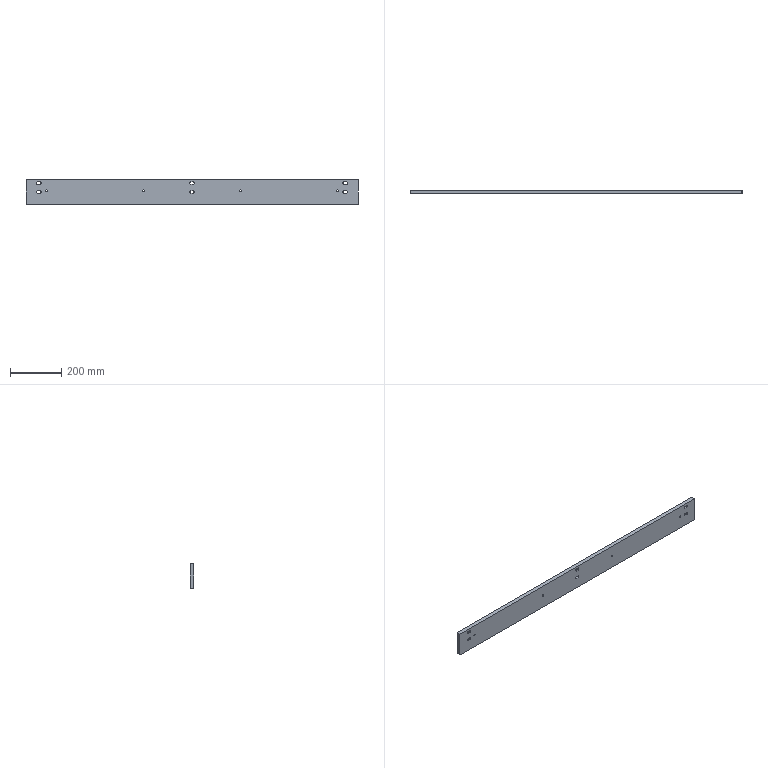Part | NX | features BREP 1 | 1 solid | 72 faces | box 1300 x 15 x 100 mm | volume 1925971 mm3 | plane 40 | cylinder 32 | commonest cylinder face diameters 10 x12 15 x12 6.8 x8